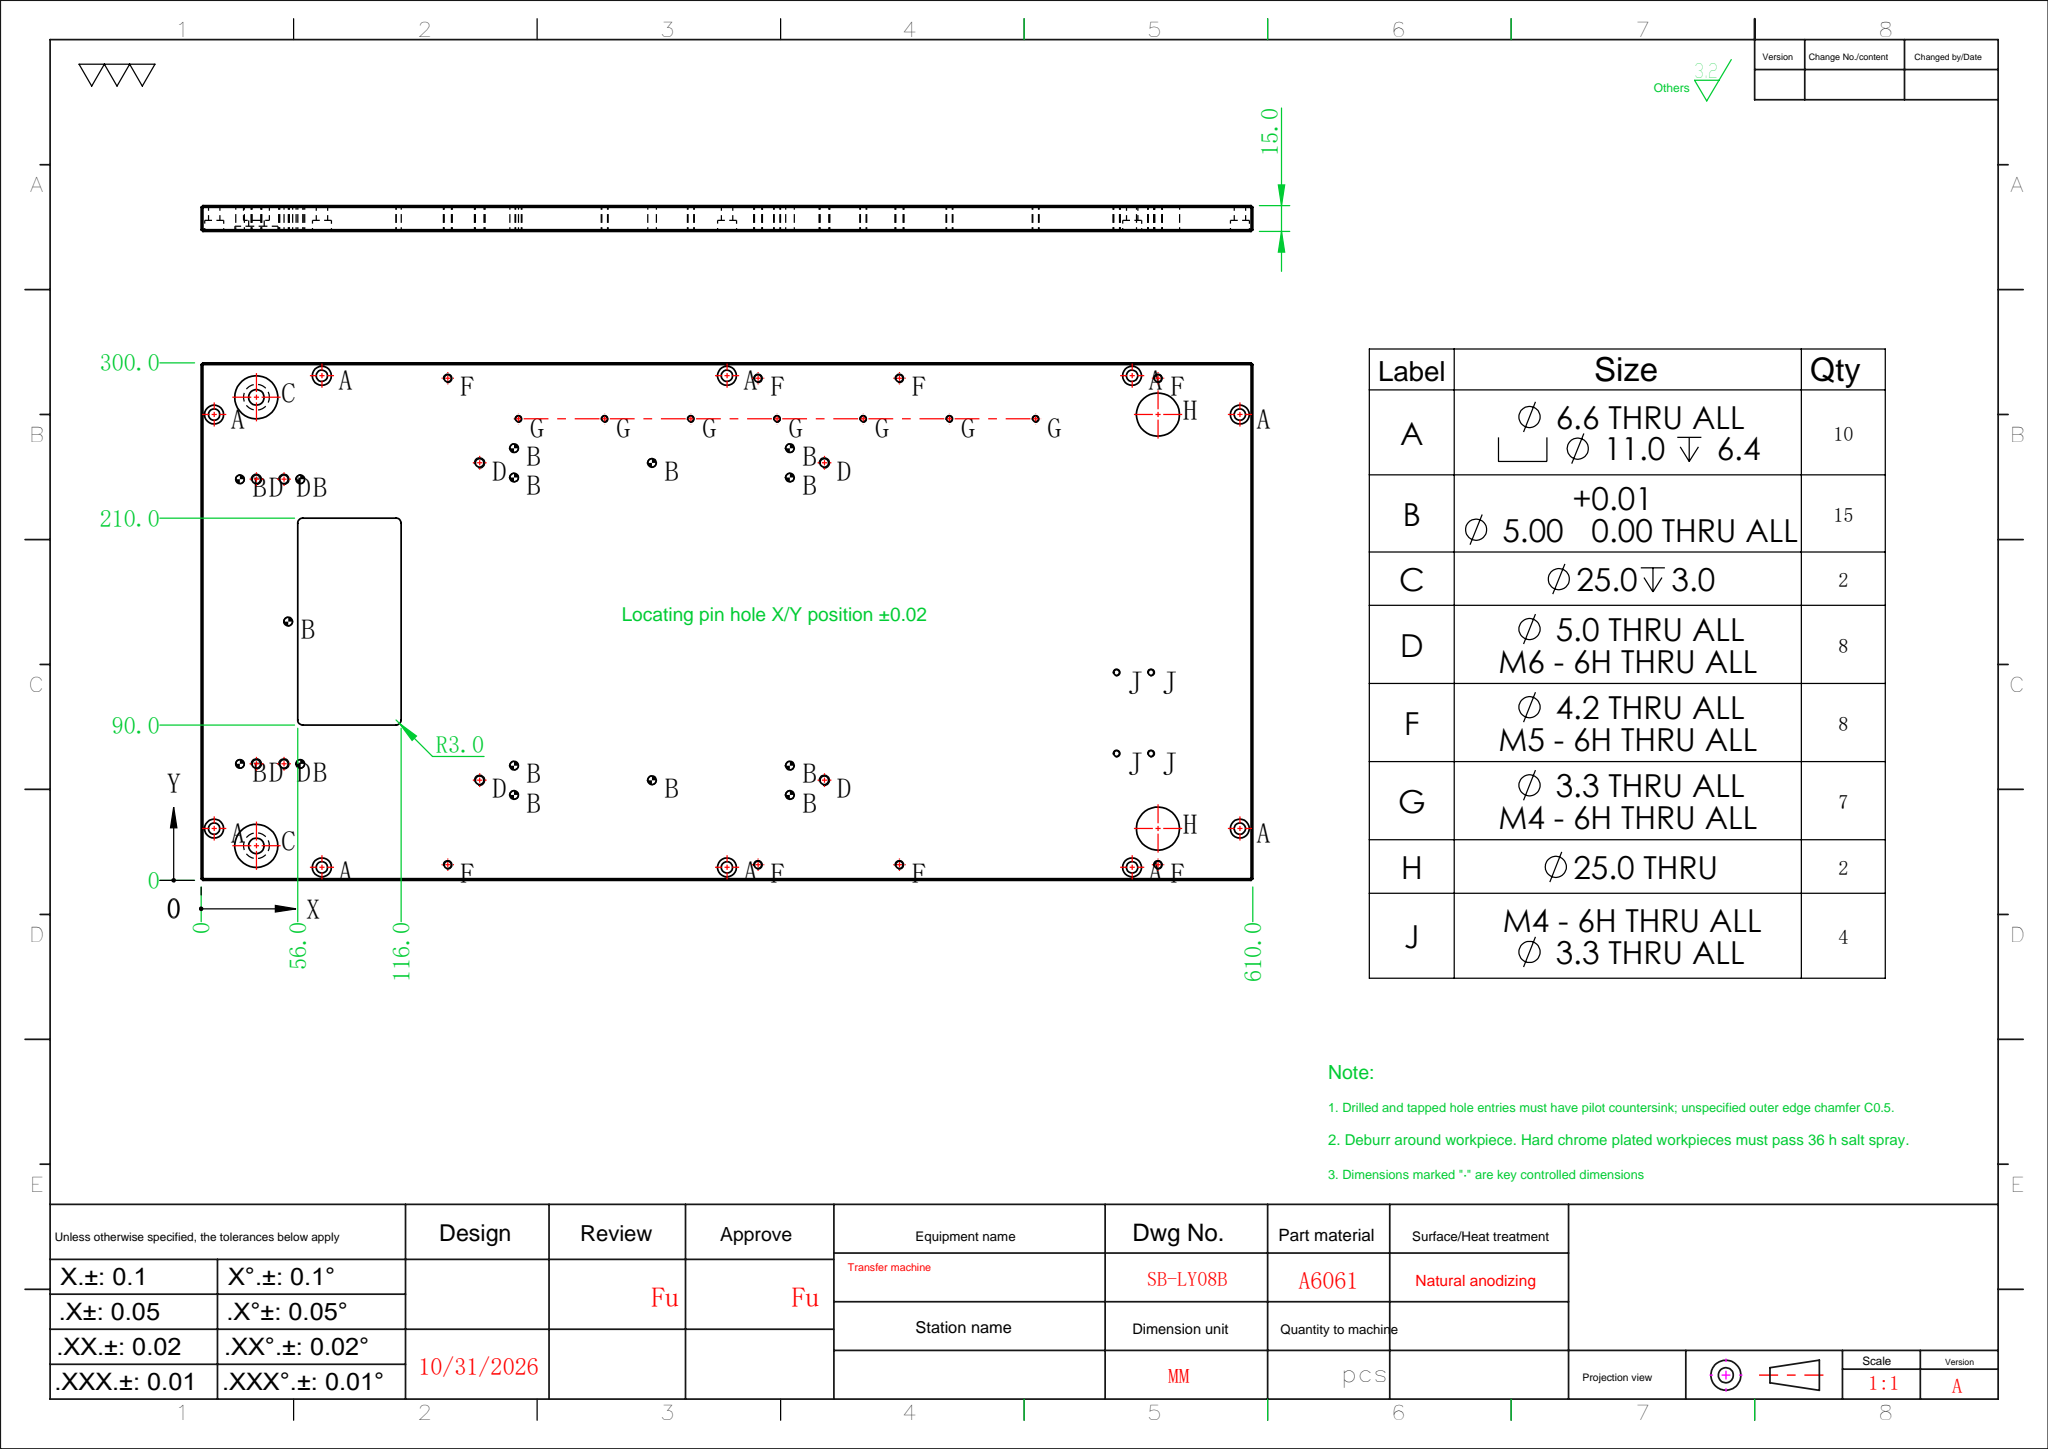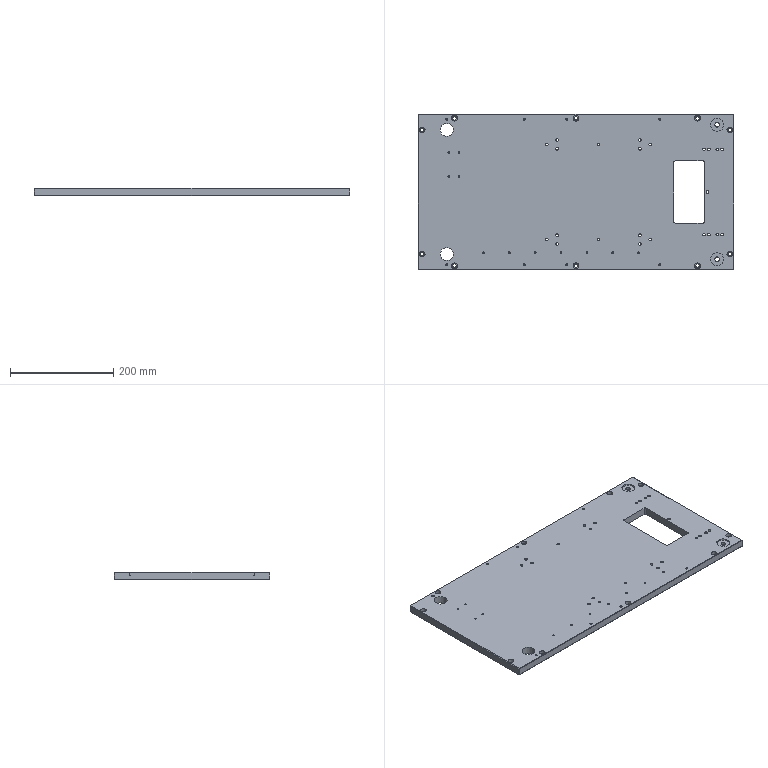Part | SolidWorks | features HoleWzd 9, Cut 3, Chamfer 1, Extrusion 1, Fillet 1, LPattern 1 | 1 solid | 188 faces | box 610 x 300 x 15 mm | volume 2595255 mm3 | cylinder 144 | plane 44 | commonest cylinder face diameters 5 x46 3.3 x22 6.6 x20 11 x20 4.2 x16 25 x8